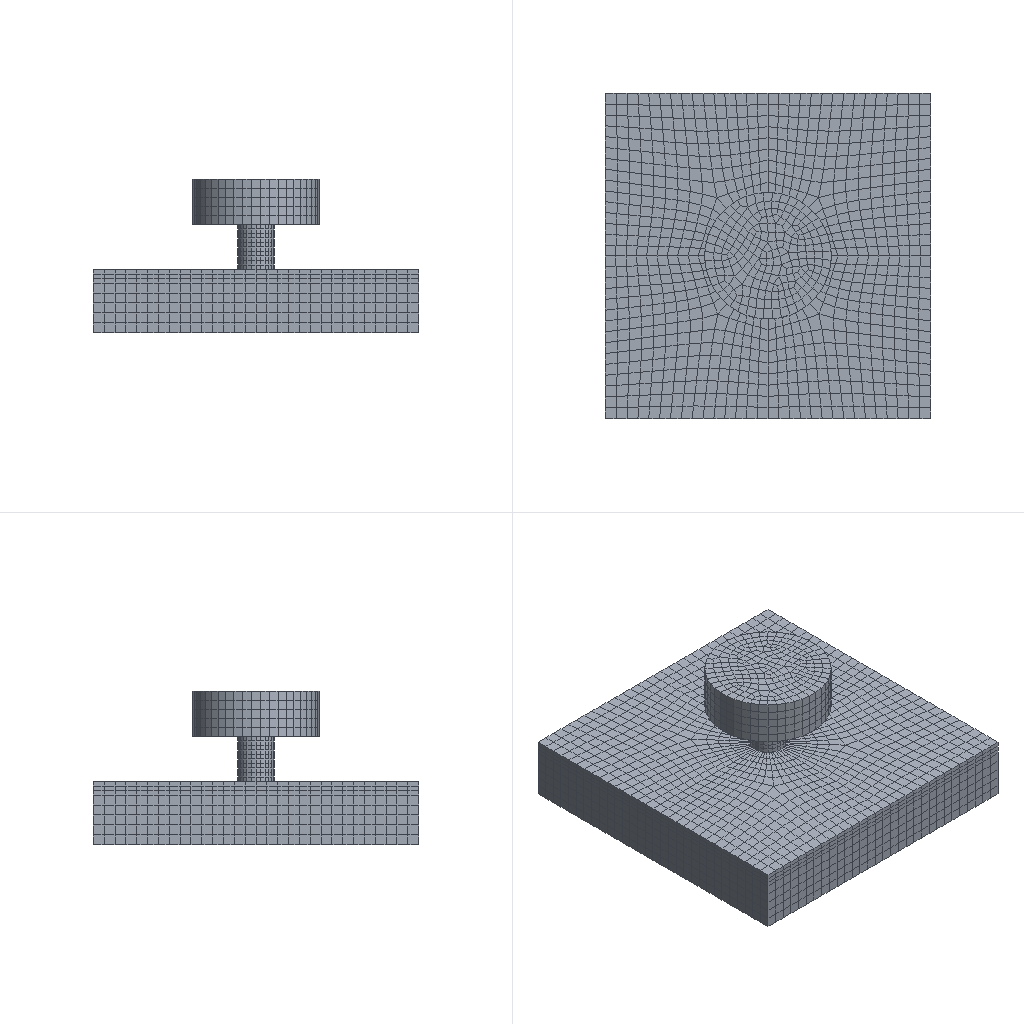Simulation study | abaqus
Set-up summary:
category,name,step,type,value,unit,region
solver,abaqus
solver,version,,,Abaqus/Standard 2020
units,not stated in the deck,,not stated
analysis,deck,,static,static
load_step,Step-load,Step-load,static
load_step,Step-1,Step-1,transient
load_step,requested,,,2
mesh,nodes,,,14226
mesh,elements,,,11492
element_type,C3D8R,,solid,11492
load,load commands in deck,,count,2
bc,support commands in deck,,count,6
material,AL2,,in results
material,AL7,,in results
material,CHUI,,in results
material,DING,,in results
check,setup vs results,,match,"per instance, exact: element labels, types and connectivity; labels of the nodes the elements use; coordinates of those nodes at SINGLE_PRECISION in 2 of 3 instance(s)"
Abaqus input file, long lists of numbers shortened:
*Heading
** Job name: Job-1 Model name: Model-1
** Generated by: Abaqus/CAE 2020
*Preprint, echo=NO, model=NO, history=NO, contact=NO
**
** PARTS
**
*Part, name=ding
*Node
      1,           2.,          6.5,           0.
      2,           2.,          4.5,           0.
** (2255 more lines like these left out)
*Element, type=C3D8R
 1,  302,  303, 1315, 1299,   20,   21,  279,  278
 2,  303,  304, 1316, 1315,   21,   22,  280,  279
** (1798 more lines like these left out)
*Nset, nset=Set-2, generate
    1,  2257,     1
*Elset, elset=Set-2, generate
    1,  1800,     1
** Section: Section-1
*Solid Section, elset=Set-2, material=ding
,
*End Part
**
*Part, name=merge
*Node
      1,          18.,         -16.,          5.5
      2,          18.,         -16.,           2.
** (10532 more lines like these left out)
*Element, type=C3D8R
   1,  941,  942, 5258, 4967,   48,   49,  812,  811
   2,  942,  943, 5259, 5258,   49,   50,  813,  812
** (8610 more lines like these left out)
*Nset, nset=Set-3
     1,     5,     6,     8,     9,    14,    18,    19,    20,    21,    22,    23,    24,    26,    27,    30
    33,    34,    35,    36,    37,    38,    39,    40,    41,    42,    43,    44,    45,    46,    47,    48
** (268 more lines like these left out)
*Elset, elset=Set-3
 2819, 2820, 2821, 2822, 2823, 2824, 2825, 2826, 2827, 2828, 2829, 2830, 2831, 2832, 2833, 2834
 2835, 2836, 2837, 2838, 2839, 2840, 2841, 2842, 2843, 2844, 2845, 2846, 2847, 2848, 2849, 2850
** (184 more lines like these left out)
*Nset, nset=Set-4
    1,    2,    3,    4,    5,    6,    7,    8,    9,   10,   11,   12,   13,   14,   15,   16
   17,   18,   19,   25,   26,   27,   28,   29,   30,   31,   32,   33,   41,   42,   43,   44
** (455 more lines like these left out)
*Elset, elset=Set-4
    1,    2,    3,    4,    5,    6,    7,    8,    9,   10,   11,   12,   13,   14,   15,   16
   17,   18,   19,   20,   21,   22,   23,   24,   25,   26,   27,   28,   29,   30,   31,   32
** (351 more lines like these left out)
** Section: Section-3
*Solid Section, elset=Set-4, material=al7
,
** Section: Section-2
*Solid Section, elset=Set-3, material=al2
,
*End Part
**
*Part, name=rigid
*Node
      1,   4.195,  -5.604,           5.
      2,   2.446,  -6.559,           5.
** (1432 more lines like these left out)
*Element, type=C3D8R
   1,  328,  339,  446,  301,   89,  100,  207,   62
   2,  436,  319,  307,  318,  197,   80,   68,   79
** (1078 more lines like these left out)
*Node
   1435,           0., -4.28626385e-16,           5.
*Nset, nset=rigid-RefPt_, internal
1435,
*Nset, nset=Set-1, generate
    1,  1434,     1
*Elset, elset=Set-1, generate
    1,  1080,     1
** Section: chui
*Solid Section, elset=Set-1, material=chui
,
*End Part
**
**
** ASSEMBLY
**
*Assembly, name=Assembly
**
*Instance, name=ding-1, part=ding
         18.,         -18.,          6.5
         18.,         -18.,          6.5, 17.,         -18.,          6.5, 90.
*End Instance
**
*Instance, name=merge-1, part=merge
*End Instance
**
*Instance, name=rigid-1, part=rigid
         18.,         -18.,          12.
*End Instance
**
*Node
      1,          18.,         -18.,          12.
*Nset, nset=Set-1, instance=ding-1
    1,    3,    5,    6,    7,    9,   10,   12,   14,   20,   21,   22,   26,   27,   28,   29
   30,   41,   42,   43,   44,   45,   54,   55,   56,   60,   61,   62,   63,   64,   65,   66
** (9 more lines like these left out)
*Nset, nset=Set-1, instance=merge-1
    3,    4,   10,   11,   12,   15,   16,   17,   28,   29,   31,   32,   88,   89,   90,   91
   92,   93,   94,   95,   96,   97,   98,   99,  100,  101,  102,  103,  104,  105,  106,  107
** (59 more lines like these left out)
*Elset, elset=Set-1, instance=ding-1
    1,    2,    3,   10,   11,   12,   19,   20,   21,   39,   42,   45,   55,   56,   57,   64
   65,   66,   73,   74,   75,   84,   87,   90,   93,   96,   99,  102,  105,  108,  111,  114
** (8 more lines like these left out)
*Elset, elset=Set-1, instance=merge-1
  211,  212,  213,  214,  215,  216,  217,  218,  219,  220,  221,  222,  223,  224,  225,  226
  227,  228,  229,  230,  231,  232,  233,  234,  235,  236,  237,  238,  239,  240,  241,  242
** (54 more lines like these left out)
*Nset, nset=Set-2, instance=rigid-1
 1435,
*Nset, nset=Set-3, instance=rigid-1
 1435,
*Nset, nset=Set-5
 1,
*Nset, nset=Set-6, instance=rigid-1
 1435,
*Nset, nset=Set-8, instance=rigid-1
 1435,
*Nset, nset=m_Set-4
 1,
*Nset, nset=m_Set-7, instance=rigid-1
 1435,
*Elset, elset=_m_Surf-1_S4, internal, instance=merge-1
    5,   10,   15,   20,   25,   30,   35,   40,   45,   50,   55,   60,   65,   70,   75,   80
   85,   90,   95,  100,  105,  110,  115,  120,  123,  126,  129,  132,  135,  138,  141,  144
** (21 more lines like these left out)
*Elset, elset=_m_Surf-1_S3, internal, instance=merge-1
  121,  122,  123,  136,  137,  138,  151,  152,  153,  166,  167,  168,  181,  182,  183,  196
  197,  198,  211,  214,  217,  220,  223,  226, 1410, 1411, 1412, 1413, 1430, 1431, 1432, 1433
** (15 more lines like these left out)
*Elset, elset=_m_Surf-1_S2, internal, instance=merge-1
  469,  470,  471,  472,  473,  474,  475,  476,  477,  478,  479,  480,  481,  482,  483,  484
  485,  486,  487,  488,  489,  490,  491,  492,  493,  494,  495,  496,  609,  610,  611,  612
** (12 more lines like these left out)
*Surface, type=ELEMENT, name=m_Surf-1
_m_Surf-1_S4, S4
_m_Surf-1_S3, S3
_m_Surf-1_S2, S2
*Elset, elset=_m_Surf-3_S1, internal, instance=rigid-1, generate
  865,  1080,     1
*Surface, type=ELEMENT, name=m_Surf-3
_m_Surf-3_S1, S1
*Elset, elset=_m_Surf-7_S1, internal, instance=rigid-1, generate
  865,  1080,     1
*Surface, type=ELEMENT, name=m_Surf-7
_m_Surf-7_S1, S1
*Elset, elset=_s_Surf-1_S3, internal, instance=ding-1
   37,   38,   39,   40,   41,   42,   43,   44,   45,  118,  119,  120,  121,  122,  123,  124
  125,  126,  163,  164,  165,  166,  167,  168,  169,  170,  171,  301,  302,  303,  304,  305
** (14 more lines like these left out)
*Elset, elset=_s_Surf-1_S4, internal, instance=ding-1
   28,   29,   30,   31,   32,   33,   34,   35,   36,   46,   47,   48,   49,   50,   51,   52
   53,   54,  127,  128,  129,  130,  131,  132,  133,  134,  135,  172,  173,  174,  175,  176
** (16 more lines like these left out)
*Elset, elset=_s_Surf-1_S2, internal, instance=ding-1
   82,   83,   84,   85,   86,   87,   88,   89,   90,  871,  872,  873,  874,  875,  876,  877
  878,  879,  880,  881,  882,  883,  884,  885,  886,  887,  888,  889,  890,  891,  892,  893
** (5 more lines like these left out)
*Surface, type=ELEMENT, name=s_Surf-1
_s_Surf-1_S3, S3
_s_Surf-1_S4, S4
_s_Surf-1_S2, S2
*Elset, elset=_s_Surf-3_S3, internal, instance=ding-1
  301,  302,  303,  304,  305,  306,  307,  308,  309,  310,  311,  312,  313,  314,  315,  316
  317,  318,  319,  320,  321,  322,  323,  324,  325,  326,  327,  328,  329,  330,  451,  452
** (12 more lines like these left out)
*Elset, elset=_s_Surf-3_S4, internal, instance=ding-1
  421,  422,  423,  424,  425,  426,  427,  428,  429,  430,  431,  432,  433,  434,  435,  436
  437,  438,  439,  440,  441,  442,  443,  444,  445,  446,  447,  448,  449,  450,  550,  560
** (12 more lines like these left out)
*Elset, elset=_s_Surf-3_S2, internal, instance=ding-1
  871,  872,  873,  874,  875,  876,  877,  878,  879,  880,  881,  882,  883,  884,  885,  886
  887,  888,  889,  890,  891,  892,  893,  894,  895,  896,  897,  898,  899,  900, 1051, 1052
** (5 more lines like these left out)
*Surface, type=ELEMENT, name=s_Surf-3
_s_Surf-3_S3, S3
_s_Surf-3_S4, S4
_s_Surf-3_S2, S2
*Elset, elset=_s_Surf-5_S4, internal, instance=merge-1
 3023, 3024, 3025, 3026, 3027, 3028, 3029, 3030, 3031, 3032, 3033, 3034, 3035, 3036, 3037, 3038
 3039, 3040, 3041, 3042, 3043, 3044, 3045, 3046, 3047, 3048, 3049, 3050, 3051, 3052, 6537, 6538
** (20 more lines like these left out)
*Elset, elset=_s_Surf-5_S3, internal, instance=merge-1
 2975, 2976, 2977, 2978, 2979, 2980, 2981, 2982, 2983, 2984, 2985, 2986, 2987, 2988, 2989, 2990
 2991, 2992, 2993, 2994, 2995, 2996, 2997, 2998, 2999, 3000, 3001, 3002, 3003, 3004, 3005, 3006
** (26 more lines like these left out)
*Elset, elset=_s_Surf-5_S2, internal, instance=merge-1
 3465, 3466, 3467, 3468, 3469, 3470, 3471, 3472, 3473, 3474, 3475, 3476, 3477, 3478, 3479, 3480
 3481, 3482, 3483, 3484, 3485, 3486, 3487, 3488, 3489, 3490, 3491, 3492, 3493, 3494, 3495, 3496
** (11 more lines like these left out)
*Surface, type=ELEMENT, name=s_Surf-5
_s_Surf-5_S4, S4
_s_Surf-5_S3, S3
_s_Surf-5_S2, S2
*Elset, elset=_s_Surf-6_S3, internal, instance=ding-1
  451,  452,  453,  481,  482,  483,  511,  512,  513,  571,  581,  591,  781,  782,  783,  811
  812,  813,  841,  842,  843, 1081, 1082, 1083, 1111, 1112, 1113, 1141, 1142, 1143, 1171, 1172
** (1 more lines like these left out)
*Elset, elset=_s_Surf-6_S4, internal, instance=ding-1
  550,  560,  570,  760,  770,  780,  880,  890,  900, 1060, 1070, 1080
*Elset, elset=_s_Surf-6_S2, internal, instance=ding-1
 1441, 1442, 1443, 1444, 1445, 1446, 1447, 1448, 1449, 1531, 1532, 1533, 1561, 1562, 1563
*Surface, type=ELEMENT, name=s_Surf-6
_s_Surf-6_S3, S3
_s_Surf-6_S4, S4
_s_Surf-6_S2, S2
*Elset, elset=_s_Surf-7_S3, internal, instance=ding-1
  451,  452,  453,  481,  482,  483,  511,  512,  513,  571,  581,  591,  781,  782,  783,  811
  812,  813,  841,  842,  843, 1081, 1082, 1083, 1111, 1112, 1113, 1141, 1142, 1143, 1171, 1172
** (1 more lines like these left out)
*Elset, elset=_s_Surf-7_S4, internal, instance=ding-1
  550,  560,  570,  760,  770,  780,  880,  890,  900, 1060, 1070, 1080
*Elset, elset=_s_Surf-7_S2, internal, instance=ding-1
 1441, 1442, 1443, 1444, 1445, 1446, 1447, 1448, 1449, 1531, 1532, 1533, 1561, 1562, 1563
*Surface, type=ELEMENT, name=s_Surf-7
_s_Surf-7_S3, S3
_s_Surf-7_S4, S4
_s_Surf-7_S2, S2
*Elset, elset=_s_Surf-9_S2, internal, instance=rigid-1, generate
   1,  216,    1
*Surface, type=ELEMENT, name=s_Surf-9
_s_Surf-9_S2, S2
** Constraint: Constraint-1
*Coupling, constraint name=Constraint-1, ref node=m_Set-7, surface=s_Surf-9
*Kinematic
*End Assembly
*Amplitude, name=Amp-1
             0.,              0.,              1.,              1.
*Amplitude, name=Amp-2, definition=PERIODIC
1,            800.,              0.,              0.
             1.,              0.
*Amplitude, name=Amp-new
             0.,              0.,             0.1,             0.1,             0.2,              0.,             0.3,             0.2
            0.4,              0.,             0.5,             0.3,             0.6,              0.,             0.7,             0.4
            0.8,              0.,             0.9,             0.5,              1.,             0.3
**
** MATERIALS
**
*Material, name=al2
*Density
 2.7e-09,
*Elastic
72000., 0.33
*Plastic
250.,0.
*Material, name=al7
*Density
 2.81e-09,
*Elastic
72000., 0.32
*Plastic
503.,0.
*Material, name=chui
*Density
 8e-09,
*Elastic
194000., 0.29
*Material, name=ding
*Density
 2.8e-09,
*Elastic
72400., 0.33
*Plastic
150.,0.
**
** INTERACTION PROPERTIES
**
*Surface Interaction, name=IntProp-1
1.,
*Friction, slip tolerance=0.005
 0.2,
*Surface Behavior, pressure-overclosure=HARD
*Surface Interaction, name=IntProp-2
1.,
*Friction, slip tolerance=0.005
 0.3,
*Surface Behavior, pressure-overclosure=HARD
*Surface Interaction, name=IntProp-3
1.,
*Surface Behavior, pressure-overclosure=HARD
**
** BOUNDARY CONDITIONS
**
** Name: BC-1 Type: 对称/反对称/完全固定
*Boundary
Set-1, ENCASTRE
** Name: BC-2 Type: 位移/转角
*Boundary
Set-8, 1, 1
Set-8, 2, 2
Set-8, 4, 4
Set-8, 5, 5
Set-8, 6, 6
**
** INTERACTIONS
**
** Interaction: Int-1
*Contact Pair, interaction=IntProp-1, type=SURFACE TO SURFACE
s_Surf-1, m_Surf-1
** Interaction: Int-4
*Contact Pair, interaction=IntProp-2, type=SURFACE TO SURFACE
s_Surf-7, m_Surf-7
** ----------------------------------------------------------------
**
** STEP: Step-load
**
*Step, name=Step-load, nlgeom=YES
*Static, stabilize=0.0002, allsdtol=0.05, continue=NO
0.01, 1., 1e-05, 1.
**
** LOADS
**
** Name: Load-1   Type: Concentrated force
*Cload, amplitude=Amp-1
Set-6, 3, -200.
**
** OUTPUT REQUESTS
**
*Restart, write, frequency=0
**
** FIELD OUTPUT: F-Output-load
**
*Output, field
*Node Output
RF, RT, U, V
*Element Output, directions=YES
E, LE, MISES, NE, PE, PEEQ, PEEQT, PEMAG, S, SF, VEEQ
*Contact Output
CDISP, CSTRESS
*Output, history, frequency=0
*End Step
** ----------------------------------------------------------------
**
** STEP: Step-1
**
*Step, name=Step-1, nlgeom=YES, inc=1000
*Dynamic
0.01,1.,1e-05
**
** LOADS
**
** Name: Load-1   Type: Concentrated force
*Cload, amplitude=Amp-new
Set-6, 3, -5000.
**
** OUTPUT REQUESTS
**
*Restart, write, number interval=1, time marks=NO
**
** FIELD OUTPUT: F-Output-load
**
*Output, field, frequency=1
*Node Output
RF, RT, U, V
*Element Output, directions=YES
E, LE, MISES, NE, PE, PEEQ, PEEQT, PEMAG, S, SF, VEEQ
*Contact Output
CDISP, CSTRESS
**
** HISTORY OUTPUT: H-Output-1
**
*Output, history, variable=PRESELECT, number interval=200, time marks=NO
*End Step
Results summary:
result,step,,completed,increments=11 time=1.0/1.0
result,step,,completed,increments=39 time=1.0/1.0
result,analysis,,,transient
result,last_loadstep,,,2
result,primary field,,,U
result,reaction total,,FX,1e-06,model units
result,reaction total,,FY,0.0,model units
result,reaction total,,FZ,1536.47,model units